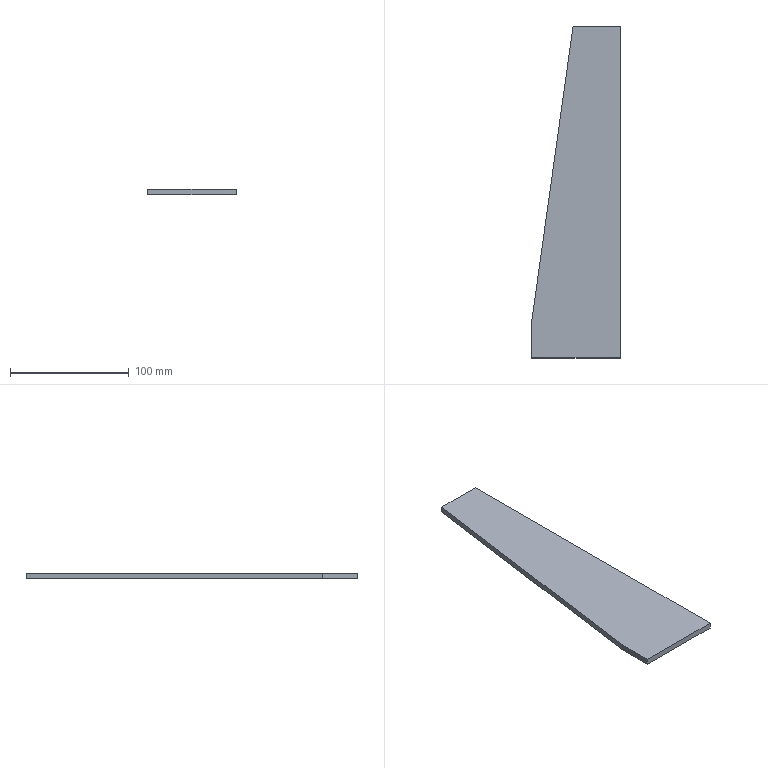Part | SolidWorks | features Extrusion 1 | 1 solid | 7 faces | box 75 x 280 x 5 mm | volume 83125 mm3 | plane 7
STEP:
#1=CARTESIAN_POINT('',(-5.,30.,0.));
#2=VERTEX_POINT('',#1);
#3=CARTESIAN_POINT('',(30.,280.,0.));
#4=VERTEX_POINT('',#3);
#5=CARTESIAN_POINT('',(-9.023,1.263,0.));
#6=DIRECTION('',(0.1386,0.9903,0.));
#7=VECTOR('',#6,1000.);
#8=LINE('',#5,#7);
#9=EDGE_CURVE('',#2,#4,#8,.T.);
#10=ORIENTED_EDGE('',*,*,#9,.F.);
#11=CARTESIAN_POINT('',(-5.,30.,5.));
#12=VERTEX_POINT('',#11);
#13=CARTESIAN_POINT('',(-5.,30.,5.));
#14=DIRECTION('',(0.,0.,-1.));
#15=VECTOR('',#14,1000.);
#16=LINE('',#13,#15);
#17=EDGE_CURVE('',#12,#2,#16,.T.);
#18=ORIENTED_EDGE('',*,*,#17,.F.);
#19=CARTESIAN_POINT('',(30.,280.,5.));
#20=VERTEX_POINT('',#19);
#21=CARTESIAN_POINT('',(-9.023,1.263,5.));
#22=DIRECTION('',(0.1386,0.9903,0.));
#23=VECTOR('',#22,1000.);
#24=LINE('',#21,#23);
#25=EDGE_CURVE('',#12,#20,#24,.T.);
#26=ORIENTED_EDGE('',*,*,#25,.T.);
#27=CARTESIAN_POINT('',(30.,280.,5.));
#28=DIRECTION('',(0.,0.,-1.));
#29=VECTOR('',#28,1000.);
#30=LINE('',#27,#29);
#31=EDGE_CURVE('',#20,#4,#30,.T.);
#32=ORIENTED_EDGE('',*,*,#31,.T.);
#33=EDGE_LOOP('',(#10,#18,#26,#32));
#34=FACE_OUTER_BOUND('',#33,.T.);
#35=CARTESIAN_POINT('',(-9.023,1.263,5.));
#36=DIRECTION('',(-0.9903,0.1386,0.));
#37=DIRECTION('',(-0.1386,-0.9903,0.));
#38=AXIS2_PLACEMENT_3D('',#35,#36,#37);
#39=PLANE('',#38);
#40=ADVANCED_FACE('',(#34),#39,.T.);
#41=CARTESIAN_POINT('',(-5.,0.,0.));
#42=VERTEX_POINT('',#41);
#43=CARTESIAN_POINT('',(-5.,0.,0.));
#44=DIRECTION('',(0.,1.,0.));
#45=VECTOR('',#44,1000.);
#46=LINE('',#43,#45);
#47=EDGE_CURVE('',#42,#2,#46,.T.);
#48=ORIENTED_EDGE('',*,*,#47,.F.);
#49=CARTESIAN_POINT('',(-5.,0.,5.));
#50=VERTEX_POINT('',#49);
#51=CARTESIAN_POINT('',(-5.,0.,5.));
#52=DIRECTION('',(0.,0.,-1.));
#53=VECTOR('',#52,1000.);
#54=LINE('',#51,#53);
#55=EDGE_CURVE('',#50,#42,#54,.T.);
#56=ORIENTED_EDGE('',*,*,#55,.F.);
#57=CARTESIAN_POINT('',(-5.,0.,5.));
#58=DIRECTION('',(0.,1.,0.));
#59=VECTOR('',#58,1000.);
#60=LINE('',#57,#59);
#61=EDGE_CURVE('',#50,#12,#60,.T.);
#62=ORIENTED_EDGE('',*,*,#61,.T.);
#63=ORIENTED_EDGE('',*,*,#17,.T.);
#64=EDGE_LOOP('',(#48,#56,#62,#63));
#65=FACE_OUTER_BOUND('',#64,.T.);
#66=CARTESIAN_POINT('',(-5.,0.,5.));
#67=DIRECTION('',(-1.,0.,0.));
#68=DIRECTION('',(0.,0.,1.));
#69=AXIS2_PLACEMENT_3D('',#66,#67,#68);
#70=PLANE('',#69);
#71=ADVANCED_FACE('',(#65),#70,.T.);
#72=CARTESIAN_POINT('',(70.,0.,0.));
#73=VERTEX_POINT('',#72);
#74=CARTESIAN_POINT('',(0.,0.,0.));
#75=DIRECTION('',(-1.,0.,0.));
#76=VECTOR('',#75,1000.);
#77=LINE('',#74,#76);
#78=EDGE_CURVE('',#73,#42,#77,.T.);
#79=ORIENTED_EDGE('',*,*,#78,.F.);
#80=CARTESIAN_POINT('',(70.,0.,5.));
#81=VERTEX_POINT('',#80);
#82=CARTESIAN_POINT('',(70.,0.,5.));
#83=DIRECTION('',(0.,0.,-1.));
#84=VECTOR('',#83,1000.);
#85=LINE('',#82,#84);
#86=EDGE_CURVE('',#81,#73,#85,.T.);
#87=ORIENTED_EDGE('',*,*,#86,.F.);
#88=CARTESIAN_POINT('',(0.,0.,5.));
#89=DIRECTION('',(-1.,0.,0.));
#90=VECTOR('',#89,1000.);
#91=LINE('',#88,#90);
#92=EDGE_CURVE('',#81,#50,#91,.T.);
#93=ORIENTED_EDGE('',*,*,#92,.T.);
#94=ORIENTED_EDGE('',*,*,#55,.T.);
#95=EDGE_LOOP('',(#79,#87,#93,#94));
#96=FACE_OUTER_BOUND('',#95,.T.);
#97=CARTESIAN_POINT('',(0.,0.,5.));
#98=DIRECTION('',(0.,-1.,0.));
#99=DIRECTION('',(1.,0.,0.));
#100=AXIS2_PLACEMENT_3D('',#97,#98,#99);
#101=PLANE('',#100);
#102=ADVANCED_FACE('',(#96),#101,.T.);
#103=CARTESIAN_POINT('',(70.,280.,0.));
#104=VERTEX_POINT('',#103);
#105=CARTESIAN_POINT('',(70.,0.,0.));
#106=DIRECTION('',(0.,1.,0.));
#107=VECTOR('',#106,1000.);
#108=LINE('',#105,#107);
#109=EDGE_CURVE('',#73,#104,#108,.T.);
#110=ORIENTED_EDGE('',*,*,#109,.T.);
#111=CARTESIAN_POINT('',(70.,280.,5.));
#112=VERTEX_POINT('',#111);
#113=CARTESIAN_POINT('',(70.,280.,5.));
#114=DIRECTION('',(0.,0.,-1.));
#115=VECTOR('',#114,1000.);
#116=LINE('',#113,#115);
#117=EDGE_CURVE('',#112,#104,#116,.T.);
#118=ORIENTED_EDGE('',*,*,#117,.F.);
#119=CARTESIAN_POINT('',(70.,0.,5.));
#120=DIRECTION('',(0.,1.,0.));
#121=VECTOR('',#120,1000.);
#122=LINE('',#119,#121);
#123=EDGE_CURVE('',#81,#112,#122,.T.);
#124=ORIENTED_EDGE('',*,*,#123,.F.);
#125=ORIENTED_EDGE('',*,*,#86,.T.);
#126=EDGE_LOOP('',(#110,#118,#124,#125));
#127=FACE_OUTER_BOUND('',#126,.T.);
#128=CARTESIAN_POINT('',(70.,0.,5.));
#129=DIRECTION('',(-1.,0.,0.));
#130=DIRECTION('',(0.,0.,1.));
#131=AXIS2_PLACEMENT_3D('',#128,#129,#130);
#132=PLANE('',#131);
#133=ADVANCED_FACE('',(#127),#132,.F.);
#134=CARTESIAN_POINT('',(0.,280.,0.));
#135=DIRECTION('',(-1.,0.,0.));
#136=VECTOR('',#135,1000.);
#137=LINE('',#134,#136);
#138=EDGE_CURVE('',#104,#4,#137,.T.);
#139=ORIENTED_EDGE('',*,*,#138,.T.);
#140=ORIENTED_EDGE('',*,*,#31,.F.);
#141=CARTESIAN_POINT('',(0.,280.,5.));
#142=DIRECTION('',(-1.,0.,0.));
#143=VECTOR('',#142,1000.);
#144=LINE('',#141,#143);
#145=EDGE_CURVE('',#112,#20,#144,.T.);
#146=ORIENTED_EDGE('',*,*,#145,.F.);
#147=ORIENTED_EDGE('',*,*,#117,.T.);
#148=EDGE_LOOP('',(#139,#140,#146,#147));
#149=FACE_OUTER_BOUND('',#148,.T.);
#150=CARTESIAN_POINT('',(0.,280.,5.));
#151=DIRECTION('',(0.,-1.,0.));
#152=DIRECTION('',(0.,0.,-1.));
#153=AXIS2_PLACEMENT_3D('',#150,#151,#152);
#154=PLANE('',#153);
#155=ADVANCED_FACE('',(#149),#154,.F.);
#156=ORIENTED_EDGE('',*,*,#25,.F.);
#157=ORIENTED_EDGE('',*,*,#61,.F.);
#158=ORIENTED_EDGE('',*,*,#92,.F.);
#159=ORIENTED_EDGE('',*,*,#123,.T.);
#160=ORIENTED_EDGE('',*,*,#145,.T.);
#161=EDGE_LOOP('',(#156,#157,#158,#159,#160));
#162=FACE_OUTER_BOUND('',#161,.T.);
#163=CARTESIAN_POINT('',(0.,0.,5.));
#164=DIRECTION('',(0.,0.,1.));
#165=DIRECTION('',(1.,0.,0.));
#166=AXIS2_PLACEMENT_3D('',#163,#164,#165);
#167=PLANE('',#166);
#168=ADVANCED_FACE('',(#162),#167,.T.);
#169=ORIENTED_EDGE('',*,*,#9,.T.);
#170=ORIENTED_EDGE('',*,*,#138,.F.);
#171=ORIENTED_EDGE('',*,*,#109,.F.);
#172=ORIENTED_EDGE('',*,*,#78,.T.);
#173=ORIENTED_EDGE('',*,*,#47,.T.);
#174=EDGE_LOOP('',(#169,#170,#171,#172,#173));
#175=FACE_OUTER_BOUND('',#174,.T.);
#176=CARTESIAN_POINT('',(0.,0.,0.));
#177=DIRECTION('',(0.,0.,1.));
#178=DIRECTION('',(1.,0.,0.));
#179=AXIS2_PLACEMENT_3D('',#176,#177,#178);
#180=PLANE('',#179);
#181=ADVANCED_FACE('',(#175),#180,.F.);
#182=CLOSED_SHELL('',(#40,#71,#102,#133,#155,#168,#181));
#183=MANIFOLD_SOLID_BREP('',#182);
#184=CARTESIAN_POINT('',(0.,0.,0.));
#185=DIRECTION('',(0.,0.,1.));
#186=DIRECTION('',(1.,0.,0.));
#187=AXIS2_PLACEMENT_3D('',#184,#185,#186);
#188=(LENGTH_UNIT()NAMED_UNIT(*)SI_UNIT(.MILLI.,.METRE.));
#189=UNCERTAINTY_MEASURE_WITH_UNIT(LENGTH_MEASURE(0.00001),#188,'','');
#190=(NAMED_UNIT(*)PLANE_ANGLE_UNIT()SI_UNIT($,.RADIAN.));
#191=(NAMED_UNIT(*)SI_UNIT($,.STERADIAN.)SOLID_ANGLE_UNIT());
#192=(GEOMETRIC_REPRESENTATION_CONTEXT(3)GLOBAL_UNCERTAINTY_ASSIGNED_CONTEXT((#189))GLOBAL_UNIT_ASSIGNED_CONTEXT((#188,#190,#191))REPRESENTATION_CONTEXT('',''));
#193=ADVANCED_BREP_SHAPE_REPRESENTATION('',(#183,#187),#192);